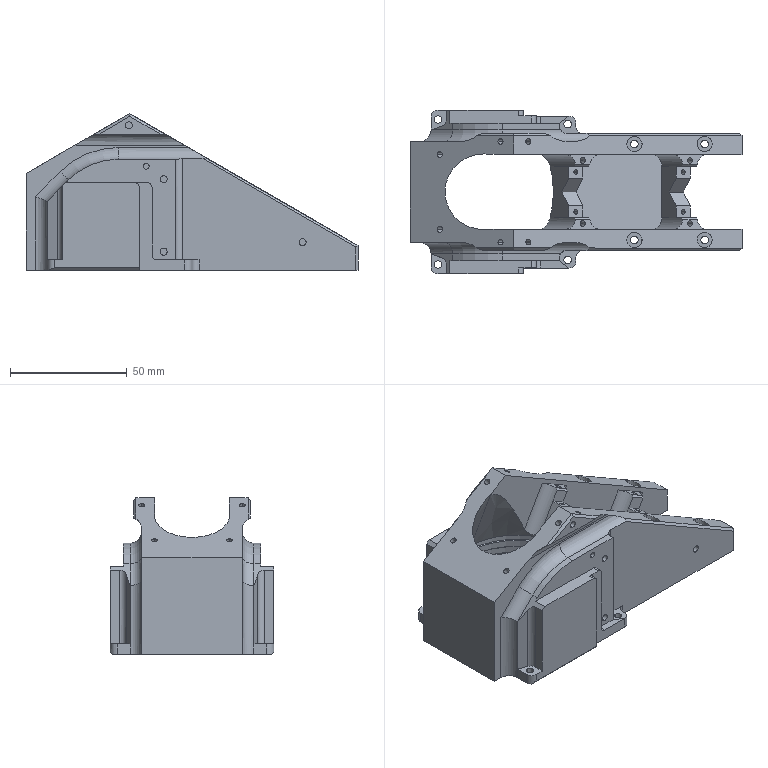Part | 1 solid | 271 faces | box 142 x 70 x 67 mm | volume 126759 mm3 | cylinder 133 | plane 126 | cone 10 | torus 2 | commonest cylinder face diameters 2.5 x24 3 x23 10 x22 3.2 x16 6 x10 2 x8